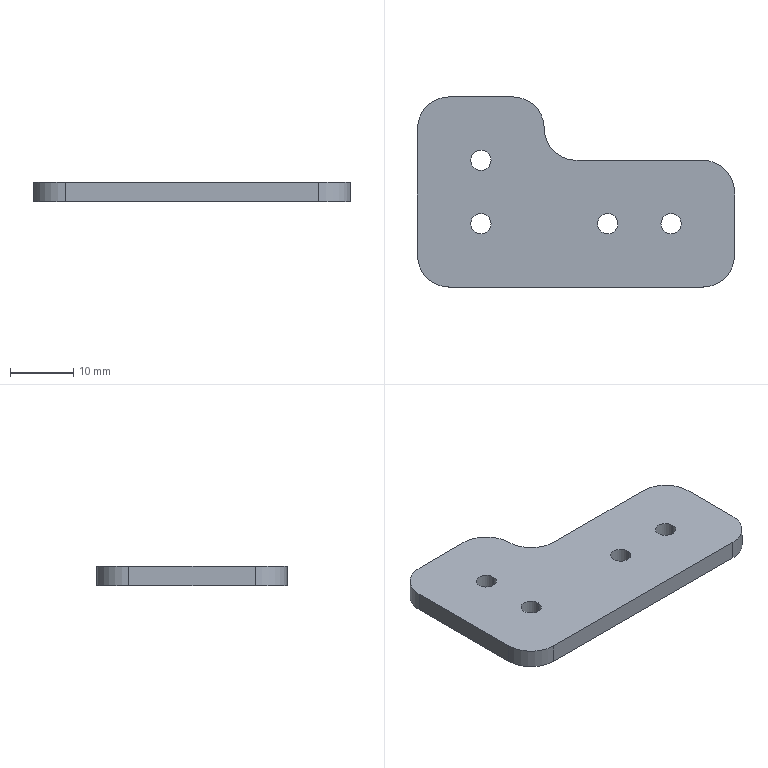Part | SolidWorks | features BaseBody 1 | 1 solid | 21 faces | box 50 x 30 x 3 mm | volume 3439 mm3 | cylinder 14 | plane 7 | commonest cylinder face diameters 3.2 x8 10 x6
STEP:
#1=CARTESIAN_POINT('',(38.4,10.,3.));
#2=VERTEX_POINT('',#1);
#3=CARTESIAN_POINT('',(41.6,10.,3.));
#4=VERTEX_POINT('',#3);
#5=CARTESIAN_POINT('',(40.,10.,3.));
#6=DIRECTION('',(0.,0.,1.));
#7=DIRECTION('',(-1.,0.,0.));
#8=AXIS2_PLACEMENT_3D('',#5,#6,#7);
#9=CIRCLE('',#8,1.6);
#10=EDGE_CURVE('',#2,#4,#9,.T.);
#11=ORIENTED_EDGE('',*,*,#10,.T.);
#12=CARTESIAN_POINT('',(41.6,10.,0.));
#13=VERTEX_POINT('',#12);
#14=CARTESIAN_POINT('',(41.6,10.,3.));
#15=DIRECTION('',(0.,0.,-1.));
#16=VECTOR('',#15,1000.);
#17=LINE('',#14,#16);
#18=EDGE_CURVE('',#4,#13,#17,.T.);
#19=ORIENTED_EDGE('',*,*,#18,.T.);
#20=CARTESIAN_POINT('',(38.4,10.,0.));
#21=VERTEX_POINT('',#20);
#22=CARTESIAN_POINT('',(40.,10.,0.));
#23=DIRECTION('',(0.,0.,1.));
#24=DIRECTION('',(-1.,0.,0.));
#25=AXIS2_PLACEMENT_3D('',#22,#23,#24);
#26=CIRCLE('',#25,1.6);
#27=EDGE_CURVE('',#21,#13,#26,.T.);
#28=ORIENTED_EDGE('',*,*,#27,.F.);
#29=CARTESIAN_POINT('',(38.4,10.,3.));
#30=DIRECTION('',(0.,0.,-1.));
#31=VECTOR('',#30,1000.);
#32=LINE('',#29,#31);
#33=EDGE_CURVE('',#2,#21,#32,.T.);
#34=ORIENTED_EDGE('',*,*,#33,.F.);
#35=EDGE_LOOP('',(#11,#19,#28,#34));
#36=FACE_OUTER_BOUND('',#35,.T.);
#37=CARTESIAN_POINT('',(40.,10.,3.));
#38=DIRECTION('',(0.,0.,-1.));
#39=DIRECTION('',(-1.,0.,0.));
#40=AXIS2_PLACEMENT_3D('',#37,#38,#39);
#41=CYLINDRICAL_SURFACE('',#40,1.6);
#42=ADVANCED_FACE('',(#36),#41,.F.);
#43=CARTESIAN_POINT('',(28.4,10.,3.));
#44=VERTEX_POINT('',#43);
#45=CARTESIAN_POINT('',(31.6,10.,3.));
#46=VERTEX_POINT('',#45);
#47=CARTESIAN_POINT('',(30.,10.,3.));
#48=DIRECTION('',(0.,0.,1.));
#49=DIRECTION('',(-1.,0.,0.));
#50=AXIS2_PLACEMENT_3D('',#47,#48,#49);
#51=CIRCLE('',#50,1.6);
#52=EDGE_CURVE('',#44,#46,#51,.T.);
#53=ORIENTED_EDGE('',*,*,#52,.T.);
#54=CARTESIAN_POINT('',(31.6,10.,0.));
#55=VERTEX_POINT('',#54);
#56=CARTESIAN_POINT('',(31.6,10.,3.));
#57=DIRECTION('',(0.,0.,-1.));
#58=VECTOR('',#57,1000.);
#59=LINE('',#56,#58);
#60=EDGE_CURVE('',#46,#55,#59,.T.);
#61=ORIENTED_EDGE('',*,*,#60,.T.);
#62=CARTESIAN_POINT('',(28.4,10.,0.));
#63=VERTEX_POINT('',#62);
#64=CARTESIAN_POINT('',(30.,10.,0.));
#65=DIRECTION('',(0.,0.,1.));
#66=DIRECTION('',(-1.,0.,0.));
#67=AXIS2_PLACEMENT_3D('',#64,#65,#66);
#68=CIRCLE('',#67,1.6);
#69=EDGE_CURVE('',#63,#55,#68,.T.);
#70=ORIENTED_EDGE('',*,*,#69,.F.);
#71=CARTESIAN_POINT('',(28.4,10.,3.));
#72=DIRECTION('',(0.,0.,-1.));
#73=VECTOR('',#72,1000.);
#74=LINE('',#71,#73);
#75=EDGE_CURVE('',#44,#63,#74,.T.);
#76=ORIENTED_EDGE('',*,*,#75,.F.);
#77=EDGE_LOOP('',(#53,#61,#70,#76));
#78=FACE_OUTER_BOUND('',#77,.T.);
#79=CARTESIAN_POINT('',(30.,10.,3.));
#80=DIRECTION('',(0.,0.,-1.));
#81=DIRECTION('',(-1.,0.,0.));
#82=AXIS2_PLACEMENT_3D('',#79,#80,#81);
#83=CYLINDRICAL_SURFACE('',#82,1.6);
#84=ADVANCED_FACE('',(#78),#83,.F.);
#85=CARTESIAN_POINT('',(8.4,10.,3.));
#86=VERTEX_POINT('',#85);
#87=CARTESIAN_POINT('',(11.6,10.,3.));
#88=VERTEX_POINT('',#87);
#89=CARTESIAN_POINT('',(10.,10.,3.));
#90=DIRECTION('',(0.,0.,1.));
#91=DIRECTION('',(-1.,0.,0.));
#92=AXIS2_PLACEMENT_3D('',#89,#90,#91);
#93=CIRCLE('',#92,1.6);
#94=EDGE_CURVE('',#86,#88,#93,.T.);
#95=ORIENTED_EDGE('',*,*,#94,.T.);
#96=CARTESIAN_POINT('',(11.6,10.,0.));
#97=VERTEX_POINT('',#96);
#98=CARTESIAN_POINT('',(11.6,10.,3.));
#99=DIRECTION('',(0.,0.,-1.));
#100=VECTOR('',#99,1000.);
#101=LINE('',#98,#100);
#102=EDGE_CURVE('',#88,#97,#101,.T.);
#103=ORIENTED_EDGE('',*,*,#102,.T.);
#104=CARTESIAN_POINT('',(8.4,10.,0.));
#105=VERTEX_POINT('',#104);
#106=CARTESIAN_POINT('',(10.,10.,0.));
#107=DIRECTION('',(0.,0.,1.));
#108=DIRECTION('',(-1.,0.,0.));
#109=AXIS2_PLACEMENT_3D('',#106,#107,#108);
#110=CIRCLE('',#109,1.6);
#111=EDGE_CURVE('',#105,#97,#110,.T.);
#112=ORIENTED_EDGE('',*,*,#111,.F.);
#113=CARTESIAN_POINT('',(8.4,10.,3.));
#114=DIRECTION('',(0.,0.,-1.));
#115=VECTOR('',#114,1000.);
#116=LINE('',#113,#115);
#117=EDGE_CURVE('',#86,#105,#116,.T.);
#118=ORIENTED_EDGE('',*,*,#117,.F.);
#119=EDGE_LOOP('',(#95,#103,#112,#118));
#120=FACE_OUTER_BOUND('',#119,.T.);
#121=CARTESIAN_POINT('',(10.,10.,3.));
#122=DIRECTION('',(0.,0.,-1.));
#123=DIRECTION('',(-1.,0.,0.));
#124=AXIS2_PLACEMENT_3D('',#121,#122,#123);
#125=CYLINDRICAL_SURFACE('',#124,1.6);
#126=ADVANCED_FACE('',(#120),#125,.F.);
#127=CARTESIAN_POINT('',(8.4,20.,3.));
#128=VERTEX_POINT('',#127);
#129=CARTESIAN_POINT('',(11.6,20.,3.));
#130=VERTEX_POINT('',#129);
#131=CARTESIAN_POINT('',(10.,20.,3.));
#132=DIRECTION('',(0.,0.,1.));
#133=DIRECTION('',(-1.,0.,0.));
#134=AXIS2_PLACEMENT_3D('',#131,#132,#133);
#135=CIRCLE('',#134,1.6);
#136=EDGE_CURVE('',#128,#130,#135,.T.);
#137=ORIENTED_EDGE('',*,*,#136,.T.);
#138=CARTESIAN_POINT('',(11.6,20.,0.));
#139=VERTEX_POINT('',#138);
#140=CARTESIAN_POINT('',(11.6,20.,3.));
#141=DIRECTION('',(0.,0.,-1.));
#142=VECTOR('',#141,1000.);
#143=LINE('',#140,#142);
#144=EDGE_CURVE('',#130,#139,#143,.T.);
#145=ORIENTED_EDGE('',*,*,#144,.T.);
#146=CARTESIAN_POINT('',(8.4,20.,0.));
#147=VERTEX_POINT('',#146);
#148=CARTESIAN_POINT('',(10.,20.,0.));
#149=DIRECTION('',(0.,0.,1.));
#150=DIRECTION('',(-1.,0.,0.));
#151=AXIS2_PLACEMENT_3D('',#148,#149,#150);
#152=CIRCLE('',#151,1.6);
#153=EDGE_CURVE('',#147,#139,#152,.T.);
#154=ORIENTED_EDGE('',*,*,#153,.F.);
#155=CARTESIAN_POINT('',(8.4,20.,3.));
#156=DIRECTION('',(0.,0.,-1.));
#157=VECTOR('',#156,1000.);
#158=LINE('',#155,#157);
#159=EDGE_CURVE('',#128,#147,#158,.T.);
#160=ORIENTED_EDGE('',*,*,#159,.F.);
#161=EDGE_LOOP('',(#137,#145,#154,#160));
#162=FACE_OUTER_BOUND('',#161,.T.);
#163=CARTESIAN_POINT('',(10.,20.,3.));
#164=DIRECTION('',(0.,0.,-1.));
#165=DIRECTION('',(-1.,0.,0.));
#166=AXIS2_PLACEMENT_3D('',#163,#164,#165);
#167=CYLINDRICAL_SURFACE('',#166,1.6);
#168=ADVANCED_FACE('',(#162),#167,.F.);
#169=ORIENTED_EDGE('',*,*,#10,.F.);
#170=CARTESIAN_POINT('',(40.,10.,3.));
#171=DIRECTION('',(0.,0.,1.));
#172=DIRECTION('',(-1.,0.,0.));
#173=AXIS2_PLACEMENT_3D('',#170,#171,#172);
#174=CIRCLE('',#173,1.6);
#175=EDGE_CURVE('',#4,#2,#174,.T.);
#176=ORIENTED_EDGE('',*,*,#175,.F.);
#177=EDGE_LOOP('',(#169,#176));
#178=FACE_BOUND('',#177,.T.);
#179=ORIENTED_EDGE('',*,*,#52,.F.);
#180=CARTESIAN_POINT('',(30.,10.,3.));
#181=DIRECTION('',(0.,0.,1.));
#182=DIRECTION('',(-1.,0.,0.));
#183=AXIS2_PLACEMENT_3D('',#180,#181,#182);
#184=CIRCLE('',#183,1.6);
#185=EDGE_CURVE('',#46,#44,#184,.T.);
#186=ORIENTED_EDGE('',*,*,#185,.F.);
#187=EDGE_LOOP('',(#179,#186));
#188=FACE_BOUND('',#187,.T.);
#189=ORIENTED_EDGE('',*,*,#94,.F.);
#190=CARTESIAN_POINT('',(10.,10.,3.));
#191=DIRECTION('',(0.,0.,1.));
#192=DIRECTION('',(-1.,0.,0.));
#193=AXIS2_PLACEMENT_3D('',#190,#191,#192);
#194=CIRCLE('',#193,1.6);
#195=EDGE_CURVE('',#88,#86,#194,.T.);
#196=ORIENTED_EDGE('',*,*,#195,.F.);
#197=EDGE_LOOP('',(#189,#196));
#198=FACE_BOUND('',#197,.T.);
#199=ORIENTED_EDGE('',*,*,#136,.F.);
#200=CARTESIAN_POINT('',(10.,20.,3.));
#201=DIRECTION('',(0.,0.,1.));
#202=DIRECTION('',(-1.,0.,0.));
#203=AXIS2_PLACEMENT_3D('',#200,#201,#202);
#204=CIRCLE('',#203,1.6);
#205=EDGE_CURVE('',#130,#128,#204,.T.);
#206=ORIENTED_EDGE('',*,*,#205,.F.);
#207=EDGE_LOOP('',(#199,#206));
#208=FACE_BOUND('',#207,.T.);
#209=CARTESIAN_POINT('',(5.,0.,3.));
#210=VERTEX_POINT('',#209);
#211=CARTESIAN_POINT('',(0.,5.,3.));
#212=VERTEX_POINT('',#211);
#213=CARTESIAN_POINT('',(5.,5.,3.));
#214=DIRECTION('',(0.,0.,-1.));
#215=DIRECTION('',(-1.,0.,0.));
#216=AXIS2_PLACEMENT_3D('',#213,#214,#215);
#217=CIRCLE('',#216,5.);
#218=EDGE_CURVE('',#210,#212,#217,.T.);
#219=ORIENTED_EDGE('',*,*,#218,.F.);
#220=CARTESIAN_POINT('',(45.,0.,3.));
#221=VERTEX_POINT('',#220);
#222=CARTESIAN_POINT('',(0.,0.,3.));
#223=DIRECTION('',(-1.,0.,0.));
#224=VECTOR('',#223,1000.);
#225=LINE('',#222,#224);
#226=EDGE_CURVE('',#221,#210,#225,.T.);
#227=ORIENTED_EDGE('',*,*,#226,.F.);
#228=CARTESIAN_POINT('',(50.,5.,3.));
#229=VERTEX_POINT('',#228);
#230=CARTESIAN_POINT('',(45.,5.,3.));
#231=DIRECTION('',(0.,0.,-1.));
#232=DIRECTION('',(-1.,0.,0.));
#233=AXIS2_PLACEMENT_3D('',#230,#231,#232);
#234=CIRCLE('',#233,5.);
#235=EDGE_CURVE('',#229,#221,#234,.T.);
#236=ORIENTED_EDGE('',*,*,#235,.F.);
#237=CARTESIAN_POINT('',(50.,15.,3.));
#238=VERTEX_POINT('',#237);
#239=CARTESIAN_POINT('',(50.,0.,3.));
#240=DIRECTION('',(0.,-1.,0.));
#241=VECTOR('',#240,1000.);
#242=LINE('',#239,#241);
#243=EDGE_CURVE('',#238,#229,#242,.T.);
#244=ORIENTED_EDGE('',*,*,#243,.F.);
#245=CARTESIAN_POINT('',(45.,20.,3.));
#246=VERTEX_POINT('',#245);
#247=CARTESIAN_POINT('',(45.,15.,3.));
#248=DIRECTION('',(0.,0.,-1.));
#249=DIRECTION('',(-1.,0.,0.));
#250=AXIS2_PLACEMENT_3D('',#247,#248,#249);
#251=CIRCLE('',#250,5.);
#252=EDGE_CURVE('',#246,#238,#251,.T.);
#253=ORIENTED_EDGE('',*,*,#252,.F.);
#254=CARTESIAN_POINT('',(25.,20.,3.));
#255=VERTEX_POINT('',#254);
#256=CARTESIAN_POINT('',(0.,20.,3.));
#257=DIRECTION('',(1.,0.,0.));
#258=VECTOR('',#257,1000.);
#259=LINE('',#256,#258);
#260=EDGE_CURVE('',#255,#246,#259,.T.);
#261=ORIENTED_EDGE('',*,*,#260,.F.);
#262=CARTESIAN_POINT('',(20.,25.,3.));
#263=VERTEX_POINT('',#262);
#264=CARTESIAN_POINT('',(25.,25.,3.));
#265=DIRECTION('',(0.,0.,1.));
#266=DIRECTION('',(1.,0.,0.));
#267=AXIS2_PLACEMENT_3D('',#264,#265,#266);
#268=CIRCLE('',#267,5.);
#269=EDGE_CURVE('',#263,#255,#268,.T.);
#270=ORIENTED_EDGE('',*,*,#269,.F.);
#271=CARTESIAN_POINT('',(15.,30.,3.));
#272=VERTEX_POINT('',#271);
#273=CARTESIAN_POINT('',(15.,25.,3.));
#274=DIRECTION('',(0.,0.,-1.));
#275=DIRECTION('',(-1.,0.,0.));
#276=AXIS2_PLACEMENT_3D('',#273,#274,#275);
#277=CIRCLE('',#276,5.);
#278=EDGE_CURVE('',#272,#263,#277,.T.);
#279=ORIENTED_EDGE('',*,*,#278,.F.);
#280=CARTESIAN_POINT('',(5.,30.,3.));
#281=VERTEX_POINT('',#280);
#282=CARTESIAN_POINT('',(0.,30.,3.));
#283=DIRECTION('',(1.,0.,0.));
#284=VECTOR('',#283,1000.);
#285=LINE('',#282,#284);
#286=EDGE_CURVE('',#281,#272,#285,.T.);
#287=ORIENTED_EDGE('',*,*,#286,.F.);
#288=CARTESIAN_POINT('',(0.,25.,3.));
#289=VERTEX_POINT('',#288);
#290=CARTESIAN_POINT('',(5.,25.,3.));
#291=DIRECTION('',(0.,0.,-1.));
#292=DIRECTION('',(-1.,0.,0.));
#293=AXIS2_PLACEMENT_3D('',#290,#291,#292);
#294=CIRCLE('',#293,5.);
#295=EDGE_CURVE('',#289,#281,#294,.T.);
#296=ORIENTED_EDGE('',*,*,#295,.F.);
#297=CARTESIAN_POINT('',(0.,0.,3.));
#298=DIRECTION('',(0.,1.,0.));
#299=VECTOR('',#298,1000.);
#300=LINE('',#297,#299);
#301=EDGE_CURVE('',#212,#289,#300,.T.);
#302=ORIENTED_EDGE('',*,*,#301,.F.);
#303=EDGE_LOOP('',(#219,#227,#236,#244,#253,#261,#270,#279,#287,#296,#302));
#304=FACE_OUTER_BOUND('',#303,.T.);
#305=CARTESIAN_POINT('',(0.,0.,3.));
#306=DIRECTION('',(0.,0.,-1.));
#307=DIRECTION('',(-1.,0.,0.));
#308=AXIS2_PLACEMENT_3D('',#305,#306,#307);
#309=PLANE('',#308);
#310=ADVANCED_FACE('',(#178,#188,#198,#208,#304),#309,.F.);
#311=ORIENTED_EDGE('',*,*,#18,.F.);
#312=ORIENTED_EDGE('',*,*,#175,.T.);
#313=ORIENTED_EDGE('',*,*,#33,.T.);
#314=CARTESIAN_POINT('',(40.,10.,0.));
#315=DIRECTION('',(0.,0.,1.));
#316=DIRECTION('',(-1.,0.,0.));
#317=AXIS2_PLACEMENT_3D('',#314,#315,#316);
#318=CIRCLE('',#317,1.6);
#319=EDGE_CURVE('',#13,#21,#318,.T.);
#320=ORIENTED_EDGE('',*,*,#319,.F.);
#321=EDGE_LOOP('',(#311,#312,#313,#320));
#322=FACE_OUTER_BOUND('',#321,.T.);
#323=CARTESIAN_POINT('',(40.,10.,3.));
#324=DIRECTION('',(0.,0.,-1.));
#325=DIRECTION('',(-1.,0.,0.));
#326=AXIS2_PLACEMENT_3D('',#323,#324,#325);
#327=CYLINDRICAL_SURFACE('',#326,1.6);
#328=ADVANCED_FACE('',(#322),#327,.F.);
#329=ORIENTED_EDGE('',*,*,#60,.F.);
#330=ORIENTED_EDGE('',*,*,#185,.T.);
#331=ORIENTED_EDGE('',*,*,#75,.T.);
#332=CARTESIAN_POINT('',(30.,10.,0.));
#333=DIRECTION('',(0.,0.,1.));
#334=DIRECTION('',(-1.,0.,0.));
#335=AXIS2_PLACEMENT_3D('',#332,#333,#334);
#336=CIRCLE('',#335,1.6);
#337=EDGE_CURVE('',#55,#63,#336,.T.);
#338=ORIENTED_EDGE('',*,*,#337,.F.);
#339=EDGE_LOOP('',(#329,#330,#331,#338));
#340=FACE_OUTER_BOUND('',#339,.T.);
#341=CARTESIAN_POINT('',(30.,10.,3.));
#342=DIRECTION('',(0.,0.,-1.));
#343=DIRECTION('',(-1.,0.,0.));
#344=AXIS2_PLACEMENT_3D('',#341,#342,#343);
#345=CYLINDRICAL_SURFACE('',#344,1.6);
#346=ADVANCED_FACE('',(#340),#345,.F.);
#347=ORIENTED_EDGE('',*,*,#102,.F.);
#348=ORIENTED_EDGE('',*,*,#195,.T.);
#349=ORIENTED_EDGE('',*,*,#117,.T.);
#350=CARTESIAN_POINT('',(10.,10.,0.));
#351=DIRECTION('',(0.,0.,1.));
#352=DIRECTION('',(-1.,0.,0.));
#353=AXIS2_PLACEMENT_3D('',#350,#351,#352);
#354=CIRCLE('',#353,1.6);
#355=EDGE_CURVE('',#97,#105,#354,.T.);
#356=ORIENTED_EDGE('',*,*,#355,.F.);
#357=EDGE_LOOP('',(#347,#348,#349,#356));
#358=FACE_OUTER_BOUND('',#357,.T.);
#359=CARTESIAN_POINT('',(10.,10.,3.));
#360=DIRECTION('',(0.,0.,-1.));
#361=DIRECTION('',(-1.,0.,0.));
#362=AXIS2_PLACEMENT_3D('',#359,#360,#361);
#363=CYLINDRICAL_SURFACE('',#362,1.6);
#364=ADVANCED_FACE('',(#358),#363,.F.);
#365=ORIENTED_EDGE('',*,*,#144,.F.);
#366=ORIENTED_EDGE('',*,*,#205,.T.);
#367=ORIENTED_EDGE('',*,*,#159,.T.);
#368=CARTESIAN_POINT('',(10.,20.,0.));
#369=DIRECTION('',(0.,0.,1.));
#370=DIRECTION('',(-1.,0.,0.));
#371=AXIS2_PLACEMENT_3D('',#368,#369,#370);
#372=CIRCLE('',#371,1.6);
#373=EDGE_CURVE('',#139,#147,#372,.T.);
#374=ORIENTED_EDGE('',*,*,#373,.F.);
#375=EDGE_LOOP('',(#365,#366,#367,#374));
#376=FACE_OUTER_BOUND('',#375,.T.);
#377=CARTESIAN_POINT('',(10.,20.,3.));
#378=DIRECTION('',(0.,0.,-1.));
#379=DIRECTION('',(-1.,0.,0.));
#380=AXIS2_PLACEMENT_3D('',#377,#378,#379);
#381=CYLINDRICAL_SURFACE('',#380,1.6);
#382=ADVANCED_FACE('',(#376),#381,.F.);
#383=CARTESIAN_POINT('',(0.,5.,0.));
#384=VERTEX_POINT('',#383);
#385=CARTESIAN_POINT('',(0.,5.,3.));
#386=DIRECTION('',(0.,0.,-1.));
#387=VECTOR('',#386,1000.);
#388=LINE('',#385,#387);
#389=EDGE_CURVE('',#212,#384,#388,.T.);
#390=ORIENTED_EDGE('',*,*,#389,.F.);
#391=ORIENTED_EDGE('',*,*,#301,.T.);
#392=CARTESIAN_POINT('',(0.,25.,0.));
#393=VERTEX_POINT('',#392);
#394=CARTESIAN_POINT('',(0.,25.,3.));
#395=DIRECTION('',(0.,0.,1.));
#396=VECTOR('',#395,1000.);
#397=LINE('',#394,#396);
#398=EDGE_CURVE('',#393,#289,#397,.T.);
#399=ORIENTED_EDGE('',*,*,#398,.F.);
#400=CARTESIAN_POINT('',(0.,0.,0.));
#401=DIRECTION('',(0.,1.,0.));
#402=VECTOR('',#401,1000.);
#403=LINE('',#400,#402);
#404=EDGE_CURVE('',#384,#393,#403,.T.);
#405=ORIENTED_EDGE('',*,*,#404,.F.);
#406=EDGE_LOOP('',(#390,#391,#399,#405));
#407=FACE_OUTER_BOUND('',#406,.T.);
#408=CARTESIAN_POINT('',(0.,0.,3.));
#409=DIRECTION('',(1.,0.,0.));
#410=DIRECTION('',(0.,1.,0.));
#411=AXIS2_PLACEMENT_3D('',#408,#409,#410);
#412=PLANE('',#411);
#413=ADVANCED_FACE('',(#407),#412,.F.);
#414=CARTESIAN_POINT('',(5.,0.,0.));
#415=VERTEX_POINT('',#414);
#416=CARTESIAN_POINT('',(5.,5.,0.));
#417=DIRECTION('',(0.,0.,1.));
#418=DIRECTION('',(-1.,0.,0.));
#419=AXIS2_PLACEMENT_3D('',#416,#417,#418);
#420=CIRCLE('',#419,5.);
#421=EDGE_CURVE('',#384,#415,#420,.T.);
#422=ORIENTED_EDGE('',*,*,#421,.T.);
#423=CARTESIAN_POINT('',(5.,0.,3.));
#424=DIRECTION('',(0.,0.,1.));
#425=VECTOR('',#424,1000.);
#426=LINE('',#423,#425);
#427=EDGE_CURVE('',#415,#210,#426,.T.);
#428=ORIENTED_EDGE('',*,*,#427,.T.);
#429=ORIENTED_EDGE('',*,*,#218,.T.);
#430=ORIENTED_EDGE('',*,*,#389,.T.);
#431=EDGE_LOOP('',(#422,#428,#429,#430));
#432=FACE_OUTER_BOUND('',#431,.T.);
#433=CARTESIAN_POINT('',(5.,5.,3.));
#434=DIRECTION('',(0.,0.,-1.));
#435=DIRECTION('',(-1.,0.,0.));
#436=AXIS2_PLACEMENT_3D('',#433,#434,#435);
#437=CYLINDRICAL_SURFACE('',#436,5.);
#438=ADVANCED_FACE('',(#432),#437,.T.);
#439=ORIENTED_EDGE('',*,*,#427,.F.);
#440=CARTESIAN_POINT('',(45.,0.,0.));
#441=VERTEX_POINT('',#440);
#442=CARTESIAN_POINT('',(50.,0.,0.));
#443=DIRECTION('',(-1.,0.,0.));
#444=VECTOR('',#443,1000.);
#445=LINE('',#442,#444);
#446=EDGE_CURVE('',#441,#415,#445,.T.);
#447=ORIENTED_EDGE('',*,*,#446,.F.);
#448=CARTESIAN_POINT('',(45.,0.,3.));
#449=DIRECTION('',(0.,0.,-1.));
#450=VECTOR('',#449,1000.);
#451=LINE('',#448,#450);
#452=EDGE_CURVE('',#221,#441,#451,.T.);
#453=ORIENTED_EDGE('',*,*,#452,.F.);
#454=ORIENTED_EDGE('',*,*,#226,.T.);
#455=EDGE_LOOP('',(#439,#447,#453,#454));
#456=FACE_OUTER_BOUND('',#455,.T.);
#457=CARTESIAN_POINT('',(50.,0.,3.));
#458=DIRECTION('',(0.,1.,0.));
#459=DIRECTION('',(-1.,0.,0.));
#460=AXIS2_PLACEMENT_3D('',#457,#458,#459);
#461=PLANE('',#460);
#462=ADVANCED_FACE('',(#456),#461,.F.);
#463=CARTESIAN_POINT('',(50.,5.,0.));
#464=VERTEX_POINT('',#463);
#465=CARTESIAN_POINT('',(45.,5.,0.));
#466=DIRECTION('',(0.,0.,1.));
#467=DIRECTION('',(-1.,0.,0.));
#468=AXIS2_PLACEMENT_3D('',#465,#466,#467);
#469=CIRCLE('',#468,5.);
#470=EDGE_CURVE('',#441,#464,#469,.T.);
#471=ORIENTED_EDGE('',*,*,#470,.T.);
#472=CARTESIAN_POINT('',(50.,5.,3.));
#473=DIRECTION('',(0.,0.,1.));
#474=VECTOR('',#473,1000.);
#475=LINE('',#472,#474);
#476=EDGE_CURVE('',#464,#229,#475,.T.);
#477=ORIENTED_EDGE('',*,*,#476,.T.);
#478=ORIENTED_EDGE('',*,*,#235,.T.);
#479=ORIENTED_EDGE('',*,*,#452,.T.);
#480=EDGE_LOOP('',(#471,#477,#478,#479));
#481=FACE_OUTER_BOUND('',#480,.T.);
#482=CARTESIAN_POINT('',(45.,5.,3.));
#483=DIRECTION('',(0.,0.,-1.));
#484=DIRECTION('',(-1.,0.,0.));
#485=AXIS2_PLACEMENT_3D('',#482,#483,#484);
#486=CYLINDRICAL_SURFACE('',#485,5.);
#487=ADVANCED_FACE('',(#481),#486,.T.);
#488=ORIENTED_EDGE('',*,*,#476,.F.);
#489=CARTESIAN_POINT('',(50.,15.,0.));
#490=VERTEX_POINT('',#489);
#491=CARTESIAN_POINT('',(50.,20.,0.));
#492=DIRECTION('',(0.,-1.,0.));
#493=VECTOR('',#492,1000.);
#494=LINE('',#491,#493);
#495=EDGE_CURVE('',#490,#464,#494,.T.);
#496=ORIENTED_EDGE('',*,*,#495,.F.);
#497=CARTESIAN_POINT('',(50.,15.,3.));
#498=DIRECTION('',(0.,0.,-1.));
#499=VECTOR('',#498,1000.);
#500=LINE('',#497,#499);
#501=EDGE_CURVE('',#238,#490,#500,.T.);
#502=ORIENTED_EDGE('',*,*,#501,.F.);
#503=ORIENTED_EDGE('',*,*,#243,.T.);
#504=EDGE_LOOP('',(#488,#496,#502,#503));
#505=FACE_OUTER_BOUND('',#504,.T.);
#506=CARTESIAN_POINT('',(50.,20.,3.));
#507=DIRECTION('',(-1.,0.,0.));
#508=DIRECTION('',(0.,-1.,0.));
#509=AXIS2_PLACEMENT_3D('',#506,#507,#508);
#510=PLANE('',#509);
#511=ADVANCED_FACE('',(#505),#510,.F.);
#512=CARTESIAN_POINT('',(45.,20.,0.));
#513=VERTEX_POINT('',#512);
#514=CARTESIAN_POINT('',(45.,15.,0.));
#515=DIRECTION('',(0.,0.,1.));
#516=DIRECTION('',(-1.,0.,0.));
#517=AXIS2_PLACEMENT_3D('',#514,#515,#516);
#518=CIRCLE('',#517,5.);
#519=EDGE_CURVE('',#490,#513,#518,.T.);
#520=ORIENTED_EDGE('',*,*,#519,.T.);
#521=CARTESIAN_POINT('',(45.,20.,3.));
#522=DIRECTION('',(0.,0.,1.));
#523=VECTOR('',#522,1000.);
#524=LINE('',#521,#523);
#525=EDGE_CURVE('',#513,#246,#524,.T.);
#526=ORIENTED_EDGE('',*,*,#525,.T.);
#527=ORIENTED_EDGE('',*,*,#252,.T.);
#528=ORIENTED_EDGE('',*,*,#501,.T.);
#529=EDGE_LOOP('',(#520,#526,#527,#528));
#530=FACE_OUTER_BOUND('',#529,.T.);
#531=CARTESIAN_POINT('',(45.,15.,3.));
#532=DIRECTION('',(0.,0.,-1.));
#533=DIRECTION('',(-1.,0.,0.));
#534=AXIS2_PLACEMENT_3D('',#531,#532,#533);
#535=CYLINDRICAL_SURFACE('',#534,5.);
#536=ADVANCED_FACE('',(#530),#535,.T.);
#537=ORIENTED_EDGE('',*,*,#525,.F.);
#538=CARTESIAN_POINT('',(25.,20.,0.));
#539=VERTEX_POINT('',#538);
#540=CARTESIAN_POINT('',(20.,20.,0.));
#541=DIRECTION('',(1.,0.,0.));
#542=VECTOR('',#541,1000.);
#543=LINE('',#540,#542);
#544=EDGE_CURVE('',#539,#513,#543,.T.);
#545=ORIENTED_EDGE('',*,*,#544,.F.);
#546=CARTESIAN_POINT('',(25.,20.,3.));
#547=DIRECTION('',(0.,0.,-1.));
#548=VECTOR('',#547,1000.);
#549=LINE('',#546,#548);
#550=EDGE_CURVE('',#255,#539,#549,.T.);
#551=ORIENTED_EDGE('',*,*,#550,.F.);
#552=ORIENTED_EDGE('',*,*,#260,.T.);
#553=EDGE_LOOP('',(#537,#545,#551,#552));
#554=FACE_OUTER_BOUND('',#553,.T.);
#555=CARTESIAN_POINT('',(20.,20.,3.));
#556=DIRECTION('',(0.,-1.,0.));
#557=DIRECTION('',(0.,0.,-1.));
#558=AXIS2_PLACEMENT_3D('',#555,#556,#557);
#559=PLANE('',#558);
#560=ADVANCED_FACE('',(#554),#559,.F.);
#561=ORIENTED_EDGE('',*,*,#550,.T.);
#562=CARTESIAN_POINT('',(20.,25.,0.));
#563=VERTEX_POINT('',#562);
#564=CARTESIAN_POINT('',(25.,25.,0.));
#565=DIRECTION('',(0.,0.,1.));
#566=DIRECTION('',(1.,0.,0.));
#567=AXIS2_PLACEMENT_3D('',#564,#565,#566);
#568=CIRCLE('',#567,5.);
#569=EDGE_CURVE('',#563,#539,#568,.T.);
#570=ORIENTED_EDGE('',*,*,#569,.F.);
#571=CARTESIAN_POINT('',(20.,25.,3.));
#572=DIRECTION('',(0.,0.,-1.));
#573=VECTOR('',#572,1000.);
#574=LINE('',#571,#573);
#575=EDGE_CURVE('',#263,#563,#574,.T.);
#576=ORIENTED_EDGE('',*,*,#575,.F.);
#577=ORIENTED_EDGE('',*,*,#269,.T.);
#578=EDGE_LOOP('',(#561,#570,#576,#577));
#579=FACE_OUTER_BOUND('',#578,.T.);
#580=CARTESIAN_POINT('',(25.,25.,3.));
#581=DIRECTION('',(0.,0.,1.));
#582=DIRECTION('',(1.,0.,0.));
#583=AXIS2_PLACEMENT_3D('',#580,#581,#582);
#584=CYLINDRICAL_SURFACE('',#583,5.);
#585=ADVANCED_FACE('',(#579),#584,.F.);
#586=ORIENTED_EDGE('',*,*,#575,.T.);
#587=CARTESIAN_POINT('',(15.,30.,0.));
#588=VERTEX_POINT('',#587);
#589=CARTESIAN_POINT('',(15.,25.,0.));
#590=DIRECTION('',(0.,0.,1.));
#591=DIRECTION('',(-1.,0.,0.));
#592=AXIS2_PLACEMENT_3D('',#589,#590,#591);
#593=CIRCLE('',#592,5.);
#594=EDGE_CURVE('',#563,#588,#593,.T.);
#595=ORIENTED_EDGE('',*,*,#594,.T.);
#596=CARTESIAN_POINT('',(15.,30.,3.));
#597=DIRECTION('',(0.,0.,1.));
#598=VECTOR('',#597,1000.);
#599=LINE('',#596,#598);
#600=EDGE_CURVE('',#588,#272,#599,.T.);
#601=ORIENTED_EDGE('',*,*,#600,.T.);
#602=ORIENTED_EDGE('',*,*,#278,.T.);
#603=EDGE_LOOP('',(#586,#595,#601,#602));
#604=FACE_OUTER_BOUND('',#603,.T.);
#605=CARTESIAN_POINT('',(15.,25.,3.));
#606=DIRECTION('',(0.,0.,-1.));
#607=DIRECTION('',(-1.,0.,0.));
#608=AXIS2_PLACEMENT_3D('',#605,#606,#607);
#609=CYLINDRICAL_SURFACE('',#608,5.);
#610=ADVANCED_FACE('',(#604),#609,.T.);
#611=ORIENTED_EDGE('',*,*,#600,.F.);
#612=CARTESIAN_POINT('',(5.,30.,0.));
#613=VERTEX_POINT('',#612);
#614=CARTESIAN_POINT('',(0.,30.,0.));
#615=DIRECTION('',(1.,0.,0.));
#616=VECTOR('',#615,1000.);
#617=LINE('',#614,#616);
#618=EDGE_CURVE('',#613,#588,#617,.T.);
#619=ORIENTED_EDGE('',*,*,#618,.F.);
#620=CARTESIAN_POINT('',(5.,30.,3.));
#621=DIRECTION('',(0.,0.,-1.));
#622=VECTOR('',#621,1000.);
#623=LINE('',#620,#622);
#624=EDGE_CURVE('',#281,#613,#623,.T.);
#625=ORIENTED_EDGE('',*,*,#624,.F.);
#626=ORIENTED_EDGE('',*,*,#286,.T.);
#627=EDGE_LOOP('',(#611,#619,#625,#626));
#628=FACE_OUTER_BOUND('',#627,.T.);
#629=CARTESIAN_POINT('',(0.,30.,3.));
#630=DIRECTION('',(0.,-1.,0.));
#631=DIRECTION('',(0.,0.,-1.));
#632=AXIS2_PLACEMENT_3D('',#629,#630,#631);
#633=PLANE('',#632);
#634=ADVANCED_FACE('',(#628),#633,.F.);
#635=CARTESIAN_POINT('',(5.,25.,0.));
#636=DIRECTION('',(0.,0.,1.));
#637=DIRECTION('',(-1.,0.,0.));
#638=AXIS2_PLACEMENT_3D('',#635,#636,#637);
#639=CIRCLE('',#638,5.);
#640=EDGE_CURVE('',#613,#393,#639,.T.);
#641=ORIENTED_EDGE('',*,*,#640,.T.);
#642=ORIENTED_EDGE('',*,*,#398,.T.);
#643=ORIENTED_EDGE('',*,*,#295,.T.);
#644=ORIENTED_EDGE('',*,*,#624,.T.);
#645=EDGE_LOOP('',(#641,#642,#643,#644));
#646=FACE_OUTER_BOUND('',#645,.T.);
#647=CARTESIAN_POINT('',(5.,25.,3.));
#648=DIRECTION('',(0.,0.,-1.));
#649=DIRECTION('',(-1.,0.,0.));
#650=AXIS2_PLACEMENT_3D('',#647,#648,#649);
#651=CYLINDRICAL_SURFACE('',#650,5.);
#652=ADVANCED_FACE('',(#646),#651,.T.);
#653=ORIENTED_EDGE('',*,*,#27,.T.);
#654=ORIENTED_EDGE('',*,*,#319,.T.);
#655=EDGE_LOOP('',(#653,#654));
#656=FACE_BOUND('',#655,.T.);
#657=ORIENTED_EDGE('',*,*,#111,.T.);
#658=ORIENTED_EDGE('',*,*,#355,.T.);
#659=EDGE_LOOP('',(#657,#658));
#660=FACE_BOUND('',#659,.T.);
#661=ORIENTED_EDGE('',*,*,#495,.T.);
#662=ORIENTED_EDGE('',*,*,#470,.F.);
#663=ORIENTED_EDGE('',*,*,#446,.T.);
#664=ORIENTED_EDGE('',*,*,#421,.F.);
#665=ORIENTED_EDGE('',*,*,#404,.T.);
#666=ORIENTED_EDGE('',*,*,#640,.F.);
#667=ORIENTED_EDGE('',*,*,#618,.T.);
#668=ORIENTED_EDGE('',*,*,#594,.F.);
#669=ORIENTED_EDGE('',*,*,#569,.T.);
#670=ORIENTED_EDGE('',*,*,#544,.T.);
#671=ORIENTED_EDGE('',*,*,#519,.F.);
#672=EDGE_LOOP('',(#661,#662,#663,#664,#665,#666,#667,#668,#669,#670,#671));
#673=FACE_OUTER_BOUND('',#672,.T.);
#674=ORIENTED_EDGE('',*,*,#153,.T.);
#675=ORIENTED_EDGE('',*,*,#373,.T.);
#676=EDGE_LOOP('',(#674,#675));
#677=FACE_BOUND('',#676,.T.);
#678=ORIENTED_EDGE('',*,*,#69,.T.);
#679=ORIENTED_EDGE('',*,*,#337,.T.);
#680=EDGE_LOOP('',(#678,#679));
#681=FACE_BOUND('',#680,.T.);
#682=CARTESIAN_POINT('',(0.,0.,0.));
#683=DIRECTION('',(0.,0.,-1.));
#684=DIRECTION('',(-1.,0.,0.));
#685=AXIS2_PLACEMENT_3D('',#682,#683,#684);
#686=PLANE('',#685);
#687=ADVANCED_FACE('',(#656,#660,#673,#677,#681),#686,.T.);
#688=CLOSED_SHELL('',(#42,#84,#126,#168,#310,#328,#346,#364,#382,#413,#438,#462,#487,#511,#536,#560,#585,#610,#634,#652,#687));
#689=MANIFOLD_SOLID_BREP('',#688);
#690=CARTESIAN_POINT('',(0.,0.,0.));
#691=DIRECTION('',(0.,0.,1.));
#692=DIRECTION('',(1.,0.,0.));
#693=AXIS2_PLACEMENT_3D('',#690,#691,#692);
#694=(LENGTH_UNIT()NAMED_UNIT(*)SI_UNIT(.MILLI.,.METRE.));
#695=UNCERTAINTY_MEASURE_WITH_UNIT(LENGTH_MEASURE(0.00001),#694,'','');
#696=(NAMED_UNIT(*)PLANE_ANGLE_UNIT()SI_UNIT($,.RADIAN.));
#697=(NAMED_UNIT(*)SI_UNIT($,.STERADIAN.)SOLID_ANGLE_UNIT());
#698=(GEOMETRIC_REPRESENTATION_CONTEXT(3)GLOBAL_UNCERTAINTY_ASSIGNED_CONTEXT((#695))GLOBAL_UNIT_ASSIGNED_CONTEXT((#694,#696,#697))REPRESENTATION_CONTEXT('',''));
#699=ADVANCED_BREP_SHAPE_REPRESENTATION('',(#689,#693),#698);